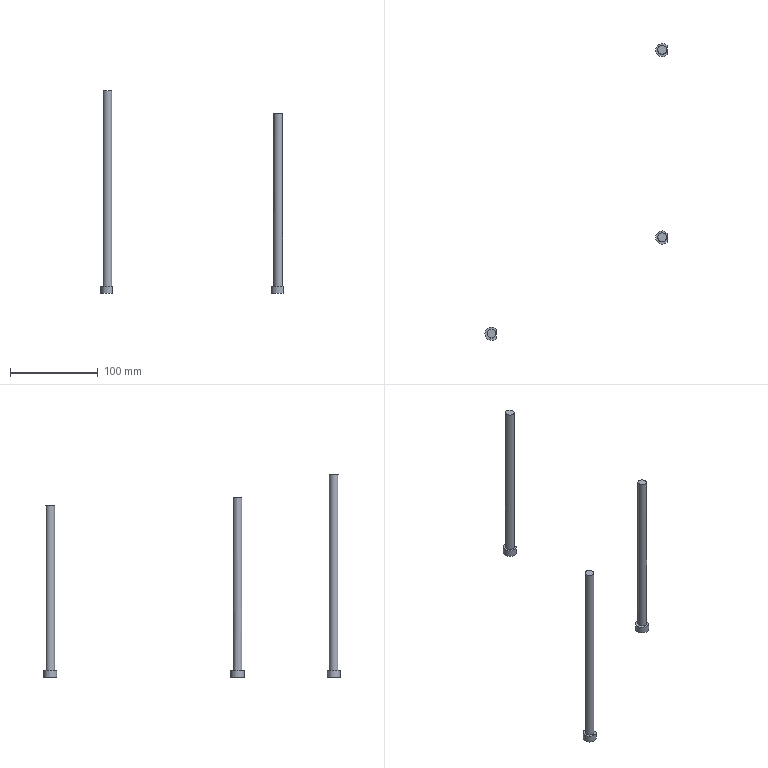Part | STEP file | DDZ10 | 3 solids | 18 faces | box 208 x 339 x 231.203 mm | volume 51713 mm3 | plane 11 | cylinder 7 | commonest cylinder face diameters 10 x3 15 x3 6922 x1